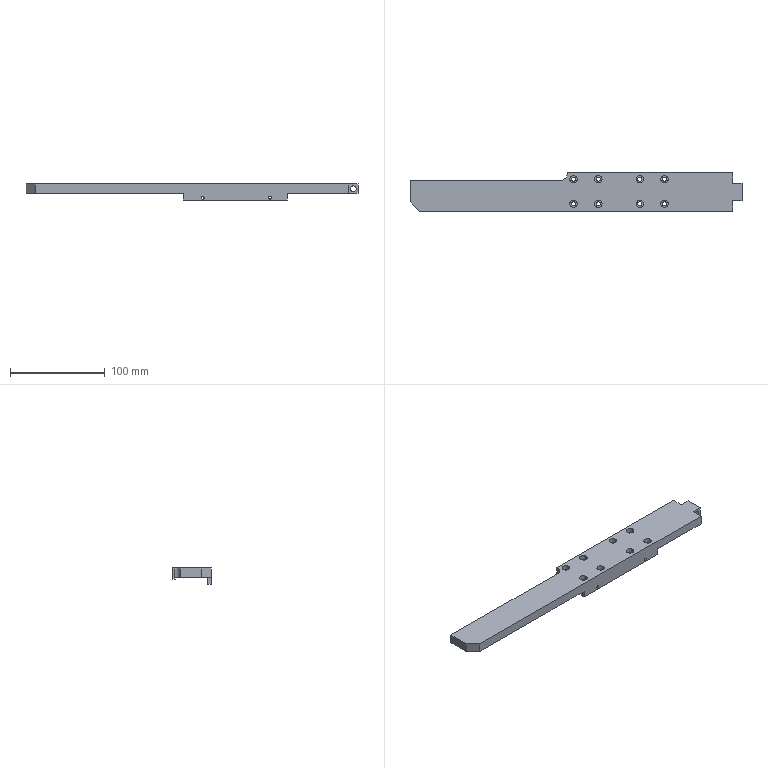Part | Creo | features CURVE 6, CUT 3, DATUM PLANE 3, PROTRUSION 3, COORDINATE SYSTEM 1 | 1 solid | 67 faces | box 350.982 x 41 x 17 mm | volume 128425 mm3 | cylinder 39 | plane 28 | commonest cylinder face diameters 4.5 x16 8 x16 3 x4 6 x2 11.655 x1